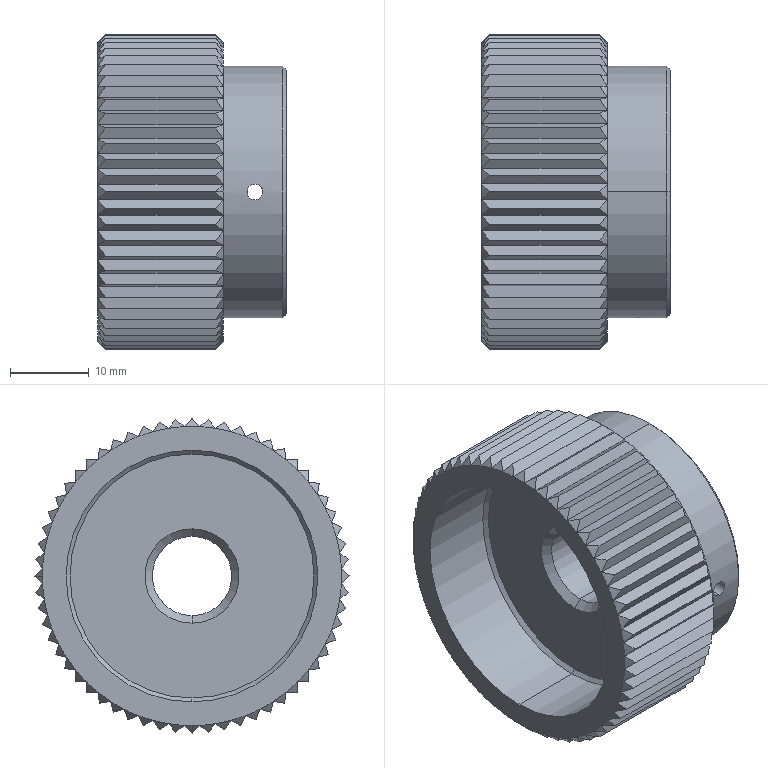Part | STEP file | KNB12_KNB12 | 1 solid | 265 faces | box 24 x 40 x 40 mm | volume 16222 mm3 | cone 131 | plane 124 | cylinder 10 | commonest cylinder face diameters 2 x4 32 x4 10.106 x2